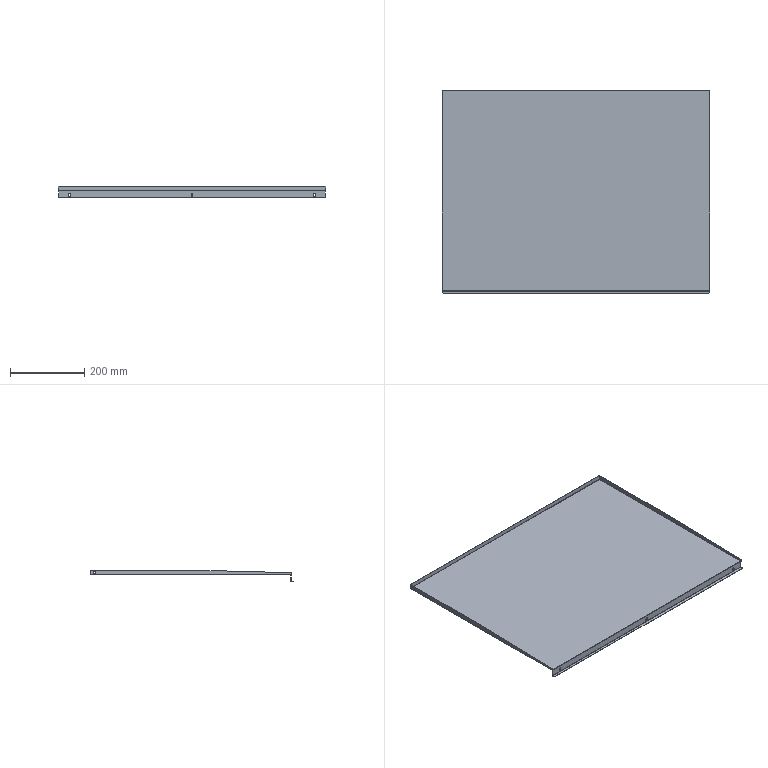Part | STEP file | RJWD-DY-0110_0002 | 1 solid | 69 faces | box 720 x 548 x 32 mm | volume 426784 mm3 | plane 42 | cylinder 23 | spline 4 | commonest cylinder face diameters 5 x6 0.4 x4 2.4 x4 6 x4 4 x2 10 x2